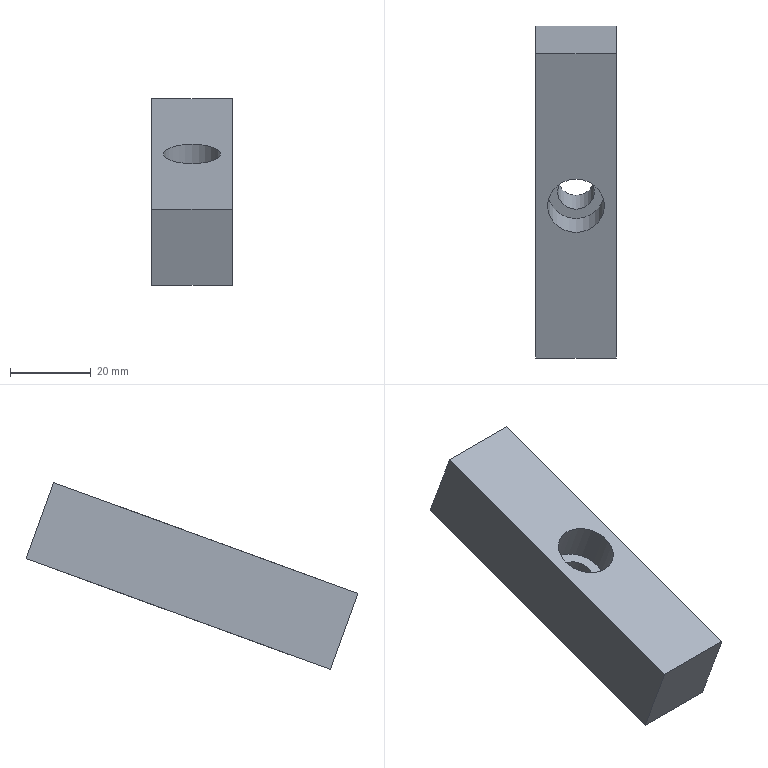Part | NX | features solid 2 | 1 solid | 9 faces | box 20 x 82.016 x 46.155 mm | volume 29824 mm3 | plane 7 | cylinder 2 | commonest cylinder face diameters 9 x1 14 x1
STEP:
#1=CARTESIAN_POINT('',(212.5,959.298,-282.517));
#2=VERTEX_POINT('',#1);
#3=CARTESIAN_POINT('',(212.5,966.138,-301.31));
#4=VERTEX_POINT('',#3);
#5=CARTESIAN_POINT('',(212.5,945.617,-244.929));
#6=DIRECTION('',(0.,0.342,-0.9397));
#7=VECTOR('',#6,1000.);
#8=LINE('',#5,#7);
#9=EDGE_CURVE('',#2,#4,#8,.T.);
#10=ORIENTED_EDGE('',*,*,#9,.F.);
#11=CARTESIAN_POINT('',(212.5,884.123,-309.878));
#12=VERTEX_POINT('',#11);
#13=CARTESIAN_POINT('',(212.5,884.123,-309.878));
#14=DIRECTION('',(0.,0.9397,0.342));
#15=VECTOR('',#14,1000.);
#16=LINE('',#13,#15);
#17=EDGE_CURVE('',#12,#2,#16,.T.);
#18=ORIENTED_EDGE('',*,*,#17,.F.);
#19=CARTESIAN_POINT('',(212.5,890.963,-328.672));
#20=VERTEX_POINT('',#19);
#21=CARTESIAN_POINT('',(212.5,870.442,-272.291));
#22=DIRECTION('',(0.,0.342,-0.9397));
#23=VECTOR('',#22,1000.);
#24=LINE('',#21,#23);
#25=EDGE_CURVE('',#12,#20,#24,.T.);
#26=ORIENTED_EDGE('',*,*,#25,.T.);
#27=CARTESIAN_POINT('',(212.5,890.963,-328.672));
#28=DIRECTION('',(0.,0.9397,0.342));
#29=VECTOR('',#28,1000.);
#30=LINE('',#27,#29);
#31=EDGE_CURVE('',#20,#4,#30,.T.);
#32=ORIENTED_EDGE('',*,*,#31,.T.);
#33=EDGE_LOOP('',(#10,#18,#26,#32));
#34=FACE_BOUND('',#33,.T.);
#35=CARTESIAN_POINT('',(212.5,870.442,-272.291));
#36=DIRECTION('',(1.,0.,0.));
#37=DIRECTION('',(0.,0.,-1.));
#38=AXIS2_PLACEMENT_3D('',#35,#36,#37);
#39=PLANE('',#38);
#40=ADVANCED_FACE('',(#34),#39,.T.);
#41=CARTESIAN_POINT('',(202.5,928.288,-293.803));
#42=VERTEX_POINT('',#41);
#43=CARTESIAN_POINT('',(202.5,921.71,-296.197));
#44=DIRECTION('',(0.,0.342,-0.9397));
#45=DIRECTION('',(0.,0.9397,0.342));
#46=AXIS2_PLACEMENT_3D('',#43,#44,#45);
#47=CIRCLE('',#46,7.);
#48=EDGE_CURVE('',#42,#42,#47,.T.);
#49=ORIENTED_EDGE('',*,*,#48,.T.);
#50=EDGE_LOOP('',(#49));
#51=FACE_BOUND('',#50,.T.);
#52=CARTESIAN_POINT('',(192.5,959.298,-282.517));
#53=VERTEX_POINT('',#52);
#54=CARTESIAN_POINT('',(192.5,959.298,-282.517));
#55=DIRECTION('',(1.,0.,0.));
#56=VECTOR('',#55,1000.);
#57=LINE('',#54,#56);
#58=EDGE_CURVE('',#53,#2,#57,.T.);
#59=ORIENTED_EDGE('',*,*,#58,.F.);
#60=CARTESIAN_POINT('',(192.5,884.123,-309.878));
#61=VERTEX_POINT('',#60);
#62=CARTESIAN_POINT('',(192.5,884.123,-309.878));
#63=DIRECTION('',(0.,0.9397,0.342));
#64=VECTOR('',#63,1000.);
#65=LINE('',#62,#64);
#66=EDGE_CURVE('',#61,#53,#65,.T.);
#67=ORIENTED_EDGE('',*,*,#66,.F.);
#68=CARTESIAN_POINT('',(192.5,884.123,-309.878));
#69=DIRECTION('',(1.,0.,0.));
#70=VECTOR('',#69,1000.);
#71=LINE('',#68,#70);
#72=EDGE_CURVE('',#61,#12,#71,.T.);
#73=ORIENTED_EDGE('',*,*,#72,.T.);
#74=ORIENTED_EDGE('',*,*,#17,.T.);
#75=EDGE_LOOP('',(#59,#67,#73,#74));
#76=FACE_BOUND('',#75,.T.);
#77=CARTESIAN_POINT('',(192.5,884.123,-309.878));
#78=DIRECTION('',(0.,-0.342,0.9397));
#79=DIRECTION('',(0.,-0.9397,-0.342));
#80=AXIS2_PLACEMENT_3D('',#77,#78,#79);
#81=PLANE('',#80);
#82=ADVANCED_FACE('',(#51,#76),#81,.T.);
#83=CARTESIAN_POINT('',(192.5,966.138,-301.31));
#84=VERTEX_POINT('',#83);
#85=CARTESIAN_POINT('',(192.5,945.617,-244.929));
#86=DIRECTION('',(0.,0.342,-0.9397));
#87=VECTOR('',#86,1000.);
#88=LINE('',#85,#87);
#89=EDGE_CURVE('',#53,#84,#88,.T.);
#90=ORIENTED_EDGE('',*,*,#89,.T.);
#91=CARTESIAN_POINT('',(192.5,890.963,-328.672));
#92=VERTEX_POINT('',#91);
#93=CARTESIAN_POINT('',(192.5,890.963,-328.672));
#94=DIRECTION('',(0.,0.9397,0.342));
#95=VECTOR('',#94,1000.);
#96=LINE('',#93,#95);
#97=EDGE_CURVE('',#92,#84,#96,.T.);
#98=ORIENTED_EDGE('',*,*,#97,.F.);
#99=CARTESIAN_POINT('',(192.5,870.442,-272.291));
#100=DIRECTION('',(0.,0.342,-0.9397));
#101=VECTOR('',#100,1000.);
#102=LINE('',#99,#101);
#103=EDGE_CURVE('',#61,#92,#102,.T.);
#104=ORIENTED_EDGE('',*,*,#103,.F.);
#105=ORIENTED_EDGE('',*,*,#66,.T.);
#106=EDGE_LOOP('',(#90,#98,#104,#105));
#107=FACE_BOUND('',#106,.T.);
#108=CARTESIAN_POINT('',(192.5,870.442,-272.291));
#109=DIRECTION('',(1.,0.,0.));
#110=DIRECTION('',(0.,0.,-1.));
#111=AXIS2_PLACEMENT_3D('',#108,#109,#110);
#112=PLANE('',#111);
#113=ADVANCED_FACE('',(#107),#112,.F.);
#114=CARTESIAN_POINT('',(202.5,924.322,-316.53));
#115=VERTEX_POINT('',#114);
#116=CARTESIAN_POINT('',(202.5,928.551,-314.991));
#117=DIRECTION('',(0.,-0.342,0.9397));
#118=DIRECTION('',(0.,-0.9397,-0.342));
#119=AXIS2_PLACEMENT_3D('',#116,#117,#118);
#120=CIRCLE('',#119,4.5);
#121=EDGE_CURVE('',#115,#115,#120,.T.);
#122=ORIENTED_EDGE('',*,*,#121,.T.);
#123=EDGE_LOOP('',(#122));
#124=FACE_BOUND('',#123,.T.);
#125=CARTESIAN_POINT('',(192.5,966.138,-301.31));
#126=DIRECTION('',(1.,0.,0.));
#127=VECTOR('',#126,1000.);
#128=LINE('',#125,#127);
#129=EDGE_CURVE('',#84,#4,#128,.T.);
#130=ORIENTED_EDGE('',*,*,#129,.T.);
#131=ORIENTED_EDGE('',*,*,#31,.F.);
#132=CARTESIAN_POINT('',(192.5,890.963,-328.672));
#133=DIRECTION('',(1.,0.,0.));
#134=VECTOR('',#133,1000.);
#135=LINE('',#132,#134);
#136=EDGE_CURVE('',#92,#20,#135,.T.);
#137=ORIENTED_EDGE('',*,*,#136,.F.);
#138=ORIENTED_EDGE('',*,*,#97,.T.);
#139=EDGE_LOOP('',(#130,#131,#137,#138));
#140=FACE_BOUND('',#139,.T.);
#141=CARTESIAN_POINT('',(192.5,890.963,-328.672));
#142=DIRECTION('',(0.,-0.342,0.9397));
#143=DIRECTION('',(0.,-0.9397,-0.342));
#144=AXIS2_PLACEMENT_3D('',#141,#142,#143);
#145=PLANE('',#144);
#146=ADVANCED_FACE('',(#124,#140),#145,.F.);
#147=ORIENTED_EDGE('',*,*,#25,.F.);
#148=ORIENTED_EDGE('',*,*,#72,.F.);
#149=ORIENTED_EDGE('',*,*,#103,.T.);
#150=ORIENTED_EDGE('',*,*,#136,.T.);
#151=EDGE_LOOP('',(#147,#148,#149,#150));
#152=FACE_BOUND('',#151,.T.);
#153=CARTESIAN_POINT('',(192.5,870.442,-272.291));
#154=DIRECTION('',(0.,-0.9397,-0.342));
#155=DIRECTION('',(0.,0.342,-0.9397));
#156=AXIS2_PLACEMENT_3D('',#153,#154,#155);
#157=PLANE('',#156);
#158=ADVANCED_FACE('',(#152),#157,.T.);
#159=ORIENTED_EDGE('',*,*,#9,.T.);
#160=ORIENTED_EDGE('',*,*,#129,.F.);
#161=ORIENTED_EDGE('',*,*,#89,.F.);
#162=ORIENTED_EDGE('',*,*,#58,.T.);
#163=EDGE_LOOP('',(#159,#160,#161,#162));
#164=FACE_BOUND('',#163,.T.);
#165=CARTESIAN_POINT('',(192.5,945.617,-244.929));
#166=DIRECTION('',(0.,-0.9397,-0.342));
#167=DIRECTION('',(0.,0.342,-0.9397));
#168=AXIS2_PLACEMENT_3D('',#165,#166,#167);
#169=PLANE('',#168);
#170=ADVANCED_FACE('',(#164),#169,.F.);
#171=CARTESIAN_POINT('',(202.5,929.359,-304.055));
#172=VERTEX_POINT('',#171);
#173=CARTESIAN_POINT('',(202.5,925.131,-305.594));
#174=DIRECTION('',(0.,0.342,-0.9397));
#175=DIRECTION('',(0.,0.9397,0.342));
#176=AXIS2_PLACEMENT_3D('',#173,#174,#175);
#177=CIRCLE('',#176,4.5);
#178=EDGE_CURVE('',#172,#172,#177,.T.);
#179=ORIENTED_EDGE('',*,*,#178,.F.);
#180=EDGE_LOOP('',(#179));
#181=FACE_BOUND('',#180,.T.);
#182=ORIENTED_EDGE('',*,*,#121,.F.);
#183=EDGE_LOOP('',(#182));
#184=FACE_BOUND('',#183,.T.);
#185=CARTESIAN_POINT('',(202.5,938.811,-343.182));
#186=DIRECTION('',(0.,0.342,-0.9397));
#187=DIRECTION('',(0.,0.9397,0.342));
#188=AXIS2_PLACEMENT_3D('',#185,#186,#187);
#189=CYLINDRICAL_SURFACE('',#188,4.5);
#190=ADVANCED_FACE('',(#181,#184),#189,.F.);
#191=ORIENTED_EDGE('',*,*,#178,.T.);
#192=EDGE_LOOP('',(#191));
#193=FACE_BOUND('',#192,.T.);
#194=CARTESIAN_POINT('',(202.5,931.708,-303.2));
#195=VERTEX_POINT('',#194);
#196=CARTESIAN_POINT('',(202.5,925.131,-305.594));
#197=DIRECTION('',(0.,0.342,-0.9397));
#198=DIRECTION('',(0.,0.9397,0.342));
#199=AXIS2_PLACEMENT_3D('',#196,#197,#198);
#200=CIRCLE('',#199,7.);
#201=EDGE_CURVE('',#195,#195,#200,.T.);
#202=ORIENTED_EDGE('',*,*,#201,.F.);
#203=EDGE_LOOP('',(#202));
#204=FACE_BOUND('',#203,.T.);
#205=CARTESIAN_POINT('',(202.5,925.131,-305.594));
#206=DIRECTION('',(0.,0.342,-0.9397));
#207=DIRECTION('',(0.,0.9397,0.342));
#208=AXIS2_PLACEMENT_3D('',#205,#206,#207);
#209=PLANE('',#208);
#210=ADVANCED_FACE('',(#193,#204),#209,.F.);
#211=ORIENTED_EDGE('',*,*,#201,.T.);
#212=EDGE_LOOP('',(#211));
#213=FACE_BOUND('',#212,.T.);
#214=ORIENTED_EDGE('',*,*,#48,.F.);
#215=EDGE_LOOP('',(#214));
#216=FACE_BOUND('',#215,.T.);
#217=CARTESIAN_POINT('',(202.5,921.71,-296.197));
#218=DIRECTION('',(0.,0.342,-0.9397));
#219=DIRECTION('',(0.,0.9397,0.342));
#220=AXIS2_PLACEMENT_3D('',#217,#218,#219);
#221=CYLINDRICAL_SURFACE('',#220,7.);
#222=ADVANCED_FACE('',(#213,#216),#221,.F.);
#223=CLOSED_SHELL('',(#40,#82,#113,#146,#158,#170,#190,#210,#222));
#224=MANIFOLD_SOLID_BREP('',#223);
#225=(LENGTH_UNIT()NAMED_UNIT(*)SI_UNIT(.MILLI.,.METRE.));
#226=UNCERTAINTY_MEASURE_WITH_UNIT(LENGTH_MEASURE(0.00001),#225,'','');
#227=(NAMED_UNIT(*)PLANE_ANGLE_UNIT()SI_UNIT($,.RADIAN.));
#228=(NAMED_UNIT(*)SI_UNIT($,.STERADIAN.)SOLID_ANGLE_UNIT());
#229=(GEOMETRIC_REPRESENTATION_CONTEXT(3)GLOBAL_UNCERTAINTY_ASSIGNED_CONTEXT((#226))GLOBAL_UNIT_ASSIGNED_CONTEXT((#225,#227,#228))REPRESENTATION_CONTEXT('',''));
#230=ADVANCED_BREP_SHAPE_REPRESENTATION('',(#224),#229);